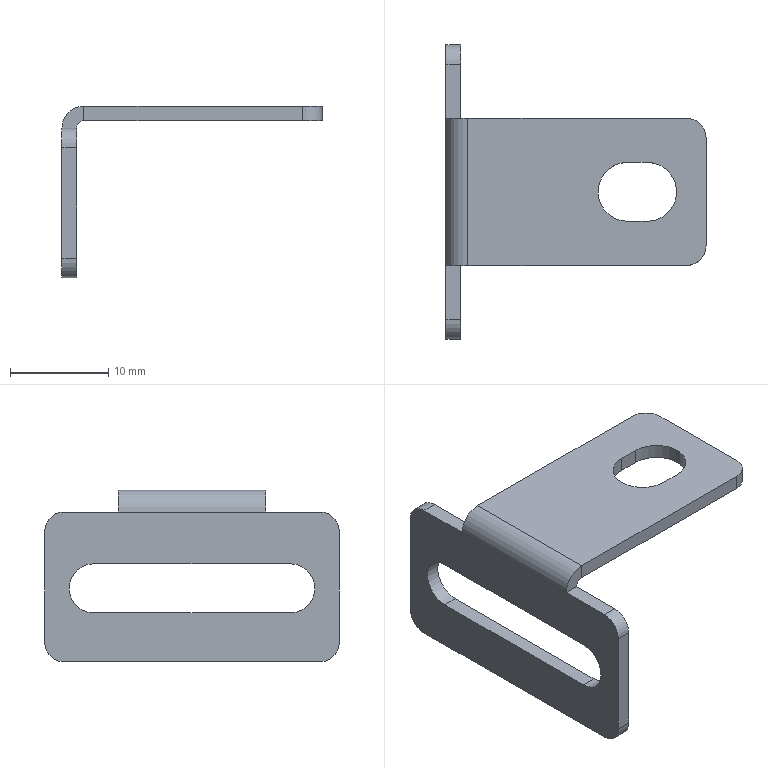Part | STEP file | b-021 | 1 solid | 31 faces | box 26.5 x 30 x 17.5 mm | volume 1038 mm3 | plane 18 | cylinder 13 | commonest cylinder face diameters 4 x6 6 x3 5 x2 1.473 x1 4.473 x1